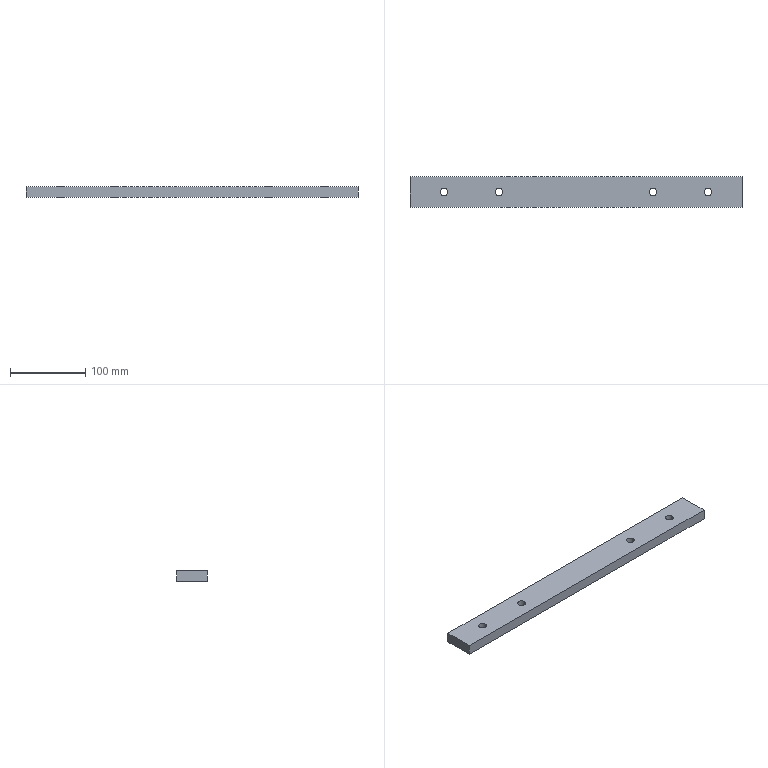Part | SolidWorks | features 3DProfileFeature 1, Extrusion 1, HoleWzd 1 | 1 solid | 14 faces | box 440 x 40 x 14 mm | volume 241824 mm3 | cylinder 8 | plane 6 | commonest cylinder face diameters 10.2 x8
STEP:
#1=CARTESIAN_POINT('',(50.1,20.,0.));
#2=VERTEX_POINT('',#1);
#3=CARTESIAN_POINT('',(39.9,20.,0.));
#4=VERTEX_POINT('',#3);
#5=CARTESIAN_POINT('',(45.,20.,0.));
#6=DIRECTION('',(0.,0.,-1.));
#7=DIRECTION('',(-1.,0.,0.));
#8=AXIS2_PLACEMENT_3D('',#5,#6,#7);
#9=CIRCLE('',#8,5.1);
#10=EDGE_CURVE('',#2,#4,#9,.T.);
#11=ORIENTED_EDGE('',*,*,#10,.T.);
#12=CARTESIAN_POINT('',(39.9,20.,14.));
#13=VERTEX_POINT('',#12);
#14=CARTESIAN_POINT('',(39.9,20.,14.));
#15=DIRECTION('',(0.,0.,1.));
#16=VECTOR('',#15,1000.);
#17=LINE('',#14,#16);
#18=EDGE_CURVE('',#4,#13,#17,.T.);
#19=ORIENTED_EDGE('',*,*,#18,.T.);
#20=CARTESIAN_POINT('',(50.1,20.,14.));
#21=VERTEX_POINT('',#20);
#22=CARTESIAN_POINT('',(45.,20.,14.));
#23=DIRECTION('',(0.,0.,1.));
#24=DIRECTION('',(1.,0.,0.));
#25=AXIS2_PLACEMENT_3D('',#22,#23,#24);
#26=CIRCLE('',#25,5.1);
#27=EDGE_CURVE('',#13,#21,#26,.T.);
#28=ORIENTED_EDGE('',*,*,#27,.T.);
#29=CARTESIAN_POINT('',(50.1,20.,14.));
#30=DIRECTION('',(0.,0.,1.));
#31=VECTOR('',#30,1000.);
#32=LINE('',#29,#31);
#33=EDGE_CURVE('',#2,#21,#32,.T.);
#34=ORIENTED_EDGE('',*,*,#33,.F.);
#35=EDGE_LOOP('',(#11,#19,#28,#34));
#36=FACE_OUTER_BOUND('',#35,.T.);
#37=CARTESIAN_POINT('',(45.,20.,14.));
#38=DIRECTION('',(0.,0.,1.));
#39=DIRECTION('',(1.,0.,0.));
#40=AXIS2_PLACEMENT_3D('',#37,#38,#39);
#41=CYLINDRICAL_SURFACE('',#40,5.1);
#42=ADVANCED_FACE('',(#36),#41,.F.);
#43=CARTESIAN_POINT('',(123.1,20.,0.));
#44=VERTEX_POINT('',#43);
#45=CARTESIAN_POINT('',(112.9,20.,0.));
#46=VERTEX_POINT('',#45);
#47=CARTESIAN_POINT('',(118.,20.,0.));
#48=DIRECTION('',(0.,0.,-1.));
#49=DIRECTION('',(-1.,0.,0.));
#50=AXIS2_PLACEMENT_3D('',#47,#48,#49);
#51=CIRCLE('',#50,5.1);
#52=EDGE_CURVE('',#44,#46,#51,.T.);
#53=ORIENTED_EDGE('',*,*,#52,.T.);
#54=CARTESIAN_POINT('',(112.9,20.,14.));
#55=VERTEX_POINT('',#54);
#56=CARTESIAN_POINT('',(112.9,20.,14.));
#57=DIRECTION('',(0.,0.,1.));
#58=VECTOR('',#57,1000.);
#59=LINE('',#56,#58);
#60=EDGE_CURVE('',#46,#55,#59,.T.);
#61=ORIENTED_EDGE('',*,*,#60,.T.);
#62=CARTESIAN_POINT('',(123.1,20.,14.));
#63=VERTEX_POINT('',#62);
#64=CARTESIAN_POINT('',(118.,20.,14.));
#65=DIRECTION('',(0.,0.,1.));
#66=DIRECTION('',(1.,0.,0.));
#67=AXIS2_PLACEMENT_3D('',#64,#65,#66);
#68=CIRCLE('',#67,5.1);
#69=EDGE_CURVE('',#55,#63,#68,.T.);
#70=ORIENTED_EDGE('',*,*,#69,.T.);
#71=CARTESIAN_POINT('',(123.1,20.,14.));
#72=DIRECTION('',(0.,0.,1.));
#73=VECTOR('',#72,1000.);
#74=LINE('',#71,#73);
#75=EDGE_CURVE('',#44,#63,#74,.T.);
#76=ORIENTED_EDGE('',*,*,#75,.F.);
#77=EDGE_LOOP('',(#53,#61,#70,#76));
#78=FACE_OUTER_BOUND('',#77,.T.);
#79=CARTESIAN_POINT('',(118.,20.,14.));
#80=DIRECTION('',(0.,0.,1.));
#81=DIRECTION('',(1.,0.,0.));
#82=AXIS2_PLACEMENT_3D('',#79,#80,#81);
#83=CYLINDRICAL_SURFACE('',#82,5.1);
#84=ADVANCED_FACE('',(#78),#83,.F.);
#85=CARTESIAN_POINT('',(400.1,20.,0.));
#86=VERTEX_POINT('',#85);
#87=CARTESIAN_POINT('',(389.9,20.,0.));
#88=VERTEX_POINT('',#87);
#89=CARTESIAN_POINT('',(395.,20.,0.));
#90=DIRECTION('',(0.,0.,-1.));
#91=DIRECTION('',(-1.,0.,0.));
#92=AXIS2_PLACEMENT_3D('',#89,#90,#91);
#93=CIRCLE('',#92,5.1);
#94=EDGE_CURVE('',#86,#88,#93,.T.);
#95=ORIENTED_EDGE('',*,*,#94,.T.);
#96=CARTESIAN_POINT('',(389.9,20.,14.));
#97=VERTEX_POINT('',#96);
#98=CARTESIAN_POINT('',(389.9,20.,14.));
#99=DIRECTION('',(0.,0.,1.));
#100=VECTOR('',#99,1000.);
#101=LINE('',#98,#100);
#102=EDGE_CURVE('',#88,#97,#101,.T.);
#103=ORIENTED_EDGE('',*,*,#102,.T.);
#104=CARTESIAN_POINT('',(400.1,20.,14.));
#105=VERTEX_POINT('',#104);
#106=CARTESIAN_POINT('',(395.,20.,14.));
#107=DIRECTION('',(0.,0.,1.));
#108=DIRECTION('',(1.,0.,0.));
#109=AXIS2_PLACEMENT_3D('',#106,#107,#108);
#110=CIRCLE('',#109,5.1);
#111=EDGE_CURVE('',#97,#105,#110,.T.);
#112=ORIENTED_EDGE('',*,*,#111,.T.);
#113=CARTESIAN_POINT('',(400.1,20.,14.));
#114=DIRECTION('',(0.,0.,1.));
#115=VECTOR('',#114,1000.);
#116=LINE('',#113,#115);
#117=EDGE_CURVE('',#86,#105,#116,.T.);
#118=ORIENTED_EDGE('',*,*,#117,.F.);
#119=EDGE_LOOP('',(#95,#103,#112,#118));
#120=FACE_OUTER_BOUND('',#119,.T.);
#121=CARTESIAN_POINT('',(395.,20.,14.));
#122=DIRECTION('',(0.,0.,1.));
#123=DIRECTION('',(1.,0.,0.));
#124=AXIS2_PLACEMENT_3D('',#121,#122,#123);
#125=CYLINDRICAL_SURFACE('',#124,5.1);
#126=ADVANCED_FACE('',(#120),#125,.F.);
#127=CARTESIAN_POINT('',(327.1,20.,0.));
#128=VERTEX_POINT('',#127);
#129=CARTESIAN_POINT('',(316.9,20.,0.));
#130=VERTEX_POINT('',#129);
#131=CARTESIAN_POINT('',(322.,20.,0.));
#132=DIRECTION('',(0.,0.,-1.));
#133=DIRECTION('',(-1.,0.,0.));
#134=AXIS2_PLACEMENT_3D('',#131,#132,#133);
#135=CIRCLE('',#134,5.1);
#136=EDGE_CURVE('',#128,#130,#135,.T.);
#137=ORIENTED_EDGE('',*,*,#136,.T.);
#138=CARTESIAN_POINT('',(316.9,20.,14.));
#139=VERTEX_POINT('',#138);
#140=CARTESIAN_POINT('',(316.9,20.,14.));
#141=DIRECTION('',(0.,0.,1.));
#142=VECTOR('',#141,1000.);
#143=LINE('',#140,#142);
#144=EDGE_CURVE('',#130,#139,#143,.T.);
#145=ORIENTED_EDGE('',*,*,#144,.T.);
#146=CARTESIAN_POINT('',(327.1,20.,14.));
#147=VERTEX_POINT('',#146);
#148=CARTESIAN_POINT('',(322.,20.,14.));
#149=DIRECTION('',(0.,0.,1.));
#150=DIRECTION('',(1.,0.,0.));
#151=AXIS2_PLACEMENT_3D('',#148,#149,#150);
#152=CIRCLE('',#151,5.1);
#153=EDGE_CURVE('',#139,#147,#152,.T.);
#154=ORIENTED_EDGE('',*,*,#153,.T.);
#155=CARTESIAN_POINT('',(327.1,20.,14.));
#156=DIRECTION('',(0.,0.,1.));
#157=VECTOR('',#156,1000.);
#158=LINE('',#155,#157);
#159=EDGE_CURVE('',#128,#147,#158,.T.);
#160=ORIENTED_EDGE('',*,*,#159,.F.);
#161=EDGE_LOOP('',(#137,#145,#154,#160));
#162=FACE_OUTER_BOUND('',#161,.T.);
#163=CARTESIAN_POINT('',(322.,20.,14.));
#164=DIRECTION('',(0.,0.,1.));
#165=DIRECTION('',(1.,0.,0.));
#166=AXIS2_PLACEMENT_3D('',#163,#164,#165);
#167=CYLINDRICAL_SURFACE('',#166,5.1);
#168=ADVANCED_FACE('',(#162),#167,.F.);
#169=CARTESIAN_POINT('',(0.,40.,0.));
#170=VERTEX_POINT('',#169);
#171=CARTESIAN_POINT('',(0.,0.,0.));
#172=VERTEX_POINT('',#171);
#173=CARTESIAN_POINT('',(0.,0.,0.));
#174=DIRECTION('',(0.,-1.,0.));
#175=VECTOR('',#174,1000.);
#176=LINE('',#173,#175);
#177=EDGE_CURVE('',#170,#172,#176,.T.);
#178=ORIENTED_EDGE('',*,*,#177,.T.);
#179=CARTESIAN_POINT('',(0.,0.,14.));
#180=VERTEX_POINT('',#179);
#181=CARTESIAN_POINT('',(0.,0.,14.));
#182=DIRECTION('',(0.,0.,-1.));
#183=VECTOR('',#182,1000.);
#184=LINE('',#181,#183);
#185=EDGE_CURVE('',#180,#172,#184,.T.);
#186=ORIENTED_EDGE('',*,*,#185,.F.);
#187=CARTESIAN_POINT('',(0.,40.,14.));
#188=VERTEX_POINT('',#187);
#189=CARTESIAN_POINT('',(0.,0.,14.));
#190=DIRECTION('',(0.,-1.,0.));
#191=VECTOR('',#190,1000.);
#192=LINE('',#189,#191);
#193=EDGE_CURVE('',#188,#180,#192,.T.);
#194=ORIENTED_EDGE('',*,*,#193,.F.);
#195=CARTESIAN_POINT('',(0.,40.,14.));
#196=DIRECTION('',(0.,0.,-1.));
#197=VECTOR('',#196,1000.);
#198=LINE('',#195,#197);
#199=EDGE_CURVE('',#188,#170,#198,.T.);
#200=ORIENTED_EDGE('',*,*,#199,.T.);
#201=EDGE_LOOP('',(#178,#186,#194,#200));
#202=FACE_OUTER_BOUND('',#201,.T.);
#203=CARTESIAN_POINT('',(0.,0.,14.));
#204=DIRECTION('',(1.,0.,0.));
#205=DIRECTION('',(0.,0.,-1.));
#206=AXIS2_PLACEMENT_3D('',#203,#204,#205);
#207=PLANE('',#206);
#208=ADVANCED_FACE('',(#202),#207,.F.);
#209=CARTESIAN_POINT('',(440.,0.,0.));
#210=VERTEX_POINT('',#209);
#211=CARTESIAN_POINT('',(0.,0.,0.));
#212=DIRECTION('',(1.,0.,0.));
#213=VECTOR('',#212,1000.);
#214=LINE('',#211,#213);
#215=EDGE_CURVE('',#172,#210,#214,.T.);
#216=ORIENTED_EDGE('',*,*,#215,.T.);
#217=CARTESIAN_POINT('',(440.,0.,14.));
#218=VERTEX_POINT('',#217);
#219=CARTESIAN_POINT('',(440.,0.,14.));
#220=DIRECTION('',(0.,0.,-1.));
#221=VECTOR('',#220,1000.);
#222=LINE('',#219,#221);
#223=EDGE_CURVE('',#218,#210,#222,.T.);
#224=ORIENTED_EDGE('',*,*,#223,.F.);
#225=CARTESIAN_POINT('',(0.,0.,14.));
#226=DIRECTION('',(1.,0.,0.));
#227=VECTOR('',#226,1000.);
#228=LINE('',#225,#227);
#229=EDGE_CURVE('',#180,#218,#228,.T.);
#230=ORIENTED_EDGE('',*,*,#229,.F.);
#231=ORIENTED_EDGE('',*,*,#185,.T.);
#232=EDGE_LOOP('',(#216,#224,#230,#231));
#233=FACE_OUTER_BOUND('',#232,.T.);
#234=CARTESIAN_POINT('',(0.,0.,14.));
#235=DIRECTION('',(0.,1.,0.));
#236=DIRECTION('',(0.,0.,1.));
#237=AXIS2_PLACEMENT_3D('',#234,#235,#236);
#238=PLANE('',#237);
#239=ADVANCED_FACE('',(#233),#238,.F.);
#240=CARTESIAN_POINT('',(440.,40.,0.));
#241=VERTEX_POINT('',#240);
#242=CARTESIAN_POINT('',(440.,0.,0.));
#243=DIRECTION('',(0.,1.,0.));
#244=VECTOR('',#243,1000.);
#245=LINE('',#242,#244);
#246=EDGE_CURVE('',#210,#241,#245,.T.);
#247=ORIENTED_EDGE('',*,*,#246,.T.);
#248=CARTESIAN_POINT('',(440.,40.,14.));
#249=VERTEX_POINT('',#248);
#250=CARTESIAN_POINT('',(440.,40.,14.));
#251=DIRECTION('',(0.,0.,-1.));
#252=VECTOR('',#251,1000.);
#253=LINE('',#250,#252);
#254=EDGE_CURVE('',#249,#241,#253,.T.);
#255=ORIENTED_EDGE('',*,*,#254,.F.);
#256=CARTESIAN_POINT('',(440.,0.,14.));
#257=DIRECTION('',(0.,1.,0.));
#258=VECTOR('',#257,1000.);
#259=LINE('',#256,#258);
#260=EDGE_CURVE('',#218,#249,#259,.T.);
#261=ORIENTED_EDGE('',*,*,#260,.F.);
#262=ORIENTED_EDGE('',*,*,#223,.T.);
#263=EDGE_LOOP('',(#247,#255,#261,#262));
#264=FACE_OUTER_BOUND('',#263,.T.);
#265=CARTESIAN_POINT('',(440.,0.,14.));
#266=DIRECTION('',(-1.,0.,0.));
#267=DIRECTION('',(0.,0.,1.));
#268=AXIS2_PLACEMENT_3D('',#265,#266,#267);
#269=PLANE('',#268);
#270=ADVANCED_FACE('',(#264),#269,.F.);
#271=CARTESIAN_POINT('',(0.,40.,0.));
#272=DIRECTION('',(-1.,0.,0.));
#273=VECTOR('',#272,1000.);
#274=LINE('',#271,#273);
#275=EDGE_CURVE('',#241,#170,#274,.T.);
#276=ORIENTED_EDGE('',*,*,#275,.T.);
#277=ORIENTED_EDGE('',*,*,#199,.F.);
#278=CARTESIAN_POINT('',(0.,40.,14.));
#279=DIRECTION('',(-1.,0.,0.));
#280=VECTOR('',#279,1000.);
#281=LINE('',#278,#280);
#282=EDGE_CURVE('',#249,#188,#281,.T.);
#283=ORIENTED_EDGE('',*,*,#282,.F.);
#284=ORIENTED_EDGE('',*,*,#254,.T.);
#285=EDGE_LOOP('',(#276,#277,#283,#284));
#286=FACE_OUTER_BOUND('',#285,.T.);
#287=CARTESIAN_POINT('',(0.,40.,14.));
#288=DIRECTION('',(0.,-1.,0.));
#289=DIRECTION('',(0.,0.,-1.));
#290=AXIS2_PLACEMENT_3D('',#287,#288,#289);
#291=PLANE('',#290);
#292=ADVANCED_FACE('',(#286),#291,.F.);
#293=CARTESIAN_POINT('',(45.,20.,14.));
#294=DIRECTION('',(0.,0.,1.));
#295=DIRECTION('',(1.,0.,0.));
#296=AXIS2_PLACEMENT_3D('',#293,#294,#295);
#297=CIRCLE('',#296,5.1);
#298=EDGE_CURVE('',#21,#13,#297,.T.);
#299=ORIENTED_EDGE('',*,*,#298,.F.);
#300=ORIENTED_EDGE('',*,*,#27,.F.);
#301=EDGE_LOOP('',(#299,#300));
#302=FACE_BOUND('',#301,.T.);
#303=CARTESIAN_POINT('',(118.,20.,14.));
#304=DIRECTION('',(0.,0.,1.));
#305=DIRECTION('',(1.,0.,0.));
#306=AXIS2_PLACEMENT_3D('',#303,#304,#305);
#307=CIRCLE('',#306,5.1);
#308=EDGE_CURVE('',#63,#55,#307,.T.);
#309=ORIENTED_EDGE('',*,*,#308,.F.);
#310=ORIENTED_EDGE('',*,*,#69,.F.);
#311=EDGE_LOOP('',(#309,#310));
#312=FACE_BOUND('',#311,.T.);
#313=CARTESIAN_POINT('',(395.,20.,14.));
#314=DIRECTION('',(0.,0.,1.));
#315=DIRECTION('',(1.,0.,0.));
#316=AXIS2_PLACEMENT_3D('',#313,#314,#315);
#317=CIRCLE('',#316,5.1);
#318=EDGE_CURVE('',#105,#97,#317,.T.);
#319=ORIENTED_EDGE('',*,*,#318,.F.);
#320=ORIENTED_EDGE('',*,*,#111,.F.);
#321=EDGE_LOOP('',(#319,#320));
#322=FACE_BOUND('',#321,.T.);
#323=CARTESIAN_POINT('',(322.,20.,14.));
#324=DIRECTION('',(0.,0.,1.));
#325=DIRECTION('',(1.,0.,0.));
#326=AXIS2_PLACEMENT_3D('',#323,#324,#325);
#327=CIRCLE('',#326,5.1);
#328=EDGE_CURVE('',#147,#139,#327,.T.);
#329=ORIENTED_EDGE('',*,*,#328,.F.);
#330=ORIENTED_EDGE('',*,*,#153,.F.);
#331=EDGE_LOOP('',(#329,#330));
#332=FACE_BOUND('',#331,.T.);
#333=ORIENTED_EDGE('',*,*,#193,.T.);
#334=ORIENTED_EDGE('',*,*,#229,.T.);
#335=ORIENTED_EDGE('',*,*,#260,.T.);
#336=ORIENTED_EDGE('',*,*,#282,.T.);
#337=EDGE_LOOP('',(#333,#334,#335,#336));
#338=FACE_OUTER_BOUND('',#337,.T.);
#339=CARTESIAN_POINT('',(0.,0.,14.));
#340=DIRECTION('',(0.,0.,-1.));
#341=DIRECTION('',(-1.,0.,0.));
#342=AXIS2_PLACEMENT_3D('',#339,#340,#341);
#343=PLANE('',#342);
#344=ADVANCED_FACE('',(#302,#312,#322,#332,#338),#343,.F.);
#345=ORIENTED_EDGE('',*,*,#10,.F.);
#346=CARTESIAN_POINT('',(45.,20.,0.));
#347=DIRECTION('',(0.,0.,-1.));
#348=DIRECTION('',(-1.,0.,0.));
#349=AXIS2_PLACEMENT_3D('',#346,#347,#348);
#350=CIRCLE('',#349,5.1);
#351=EDGE_CURVE('',#4,#2,#350,.T.);
#352=ORIENTED_EDGE('',*,*,#351,.F.);
#353=EDGE_LOOP('',(#345,#352));
#354=FACE_BOUND('',#353,.T.);
#355=ORIENTED_EDGE('',*,*,#52,.F.);
#356=CARTESIAN_POINT('',(118.,20.,0.));
#357=DIRECTION('',(0.,0.,-1.));
#358=DIRECTION('',(-1.,0.,0.));
#359=AXIS2_PLACEMENT_3D('',#356,#357,#358);
#360=CIRCLE('',#359,5.1);
#361=EDGE_CURVE('',#46,#44,#360,.T.);
#362=ORIENTED_EDGE('',*,*,#361,.F.);
#363=EDGE_LOOP('',(#355,#362));
#364=FACE_BOUND('',#363,.T.);
#365=ORIENTED_EDGE('',*,*,#94,.F.);
#366=CARTESIAN_POINT('',(395.,20.,0.));
#367=DIRECTION('',(0.,0.,-1.));
#368=DIRECTION('',(-1.,0.,0.));
#369=AXIS2_PLACEMENT_3D('',#366,#367,#368);
#370=CIRCLE('',#369,5.1);
#371=EDGE_CURVE('',#88,#86,#370,.T.);
#372=ORIENTED_EDGE('',*,*,#371,.F.);
#373=EDGE_LOOP('',(#365,#372));
#374=FACE_BOUND('',#373,.T.);
#375=ORIENTED_EDGE('',*,*,#136,.F.);
#376=CARTESIAN_POINT('',(322.,20.,0.));
#377=DIRECTION('',(0.,0.,-1.));
#378=DIRECTION('',(-1.,0.,0.));
#379=AXIS2_PLACEMENT_3D('',#376,#377,#378);
#380=CIRCLE('',#379,5.1);
#381=EDGE_CURVE('',#130,#128,#380,.T.);
#382=ORIENTED_EDGE('',*,*,#381,.F.);
#383=EDGE_LOOP('',(#375,#382));
#384=FACE_BOUND('',#383,.T.);
#385=ORIENTED_EDGE('',*,*,#177,.F.);
#386=ORIENTED_EDGE('',*,*,#275,.F.);
#387=ORIENTED_EDGE('',*,*,#246,.F.);
#388=ORIENTED_EDGE('',*,*,#215,.F.);
#389=EDGE_LOOP('',(#385,#386,#387,#388));
#390=FACE_OUTER_BOUND('',#389,.T.);
#391=CARTESIAN_POINT('',(0.,0.,0.));
#392=DIRECTION('',(0.,0.,-1.));
#393=DIRECTION('',(-1.,0.,0.));
#394=AXIS2_PLACEMENT_3D('',#391,#392,#393);
#395=PLANE('',#394);
#396=ADVANCED_FACE('',(#354,#364,#374,#384,#390),#395,.T.);
#397=ORIENTED_EDGE('',*,*,#144,.F.);
#398=ORIENTED_EDGE('',*,*,#381,.T.);
#399=ORIENTED_EDGE('',*,*,#159,.T.);
#400=ORIENTED_EDGE('',*,*,#328,.T.);
#401=EDGE_LOOP('',(#397,#398,#399,#400));
#402=FACE_OUTER_BOUND('',#401,.T.);
#403=CARTESIAN_POINT('',(322.,20.,14.));
#404=DIRECTION('',(0.,0.,1.));
#405=DIRECTION('',(1.,0.,0.));
#406=AXIS2_PLACEMENT_3D('',#403,#404,#405);
#407=CYLINDRICAL_SURFACE('',#406,5.1);
#408=ADVANCED_FACE('',(#402),#407,.F.);
#409=ORIENTED_EDGE('',*,*,#102,.F.);
#410=ORIENTED_EDGE('',*,*,#371,.T.);
#411=ORIENTED_EDGE('',*,*,#117,.T.);
#412=ORIENTED_EDGE('',*,*,#318,.T.);
#413=EDGE_LOOP('',(#409,#410,#411,#412));
#414=FACE_OUTER_BOUND('',#413,.T.);
#415=CARTESIAN_POINT('',(395.,20.,14.));
#416=DIRECTION('',(0.,0.,1.));
#417=DIRECTION('',(1.,0.,0.));
#418=AXIS2_PLACEMENT_3D('',#415,#416,#417);
#419=CYLINDRICAL_SURFACE('',#418,5.1);
#420=ADVANCED_FACE('',(#414),#419,.F.);
#421=ORIENTED_EDGE('',*,*,#60,.F.);
#422=ORIENTED_EDGE('',*,*,#361,.T.);
#423=ORIENTED_EDGE('',*,*,#75,.T.);
#424=ORIENTED_EDGE('',*,*,#308,.T.);
#425=EDGE_LOOP('',(#421,#422,#423,#424));
#426=FACE_OUTER_BOUND('',#425,.T.);
#427=CARTESIAN_POINT('',(118.,20.,14.));
#428=DIRECTION('',(0.,0.,1.));
#429=DIRECTION('',(1.,0.,0.));
#430=AXIS2_PLACEMENT_3D('',#427,#428,#429);
#431=CYLINDRICAL_SURFACE('',#430,5.1);
#432=ADVANCED_FACE('',(#426),#431,.F.);
#433=ORIENTED_EDGE('',*,*,#18,.F.);
#434=ORIENTED_EDGE('',*,*,#351,.T.);
#435=ORIENTED_EDGE('',*,*,#33,.T.);
#436=ORIENTED_EDGE('',*,*,#298,.T.);
#437=EDGE_LOOP('',(#433,#434,#435,#436));
#438=FACE_OUTER_BOUND('',#437,.T.);
#439=CARTESIAN_POINT('',(45.,20.,14.));
#440=DIRECTION('',(0.,0.,1.));
#441=DIRECTION('',(1.,0.,0.));
#442=AXIS2_PLACEMENT_3D('',#439,#440,#441);
#443=CYLINDRICAL_SURFACE('',#442,5.1);
#444=ADVANCED_FACE('',(#438),#443,.F.);
#445=CLOSED_SHELL('',(#42,#84,#126,#168,#208,#239,#270,#292,#344,#396,#408,#420,#432,#444));
#446=MANIFOLD_SOLID_BREP('',#445);
#447=CARTESIAN_POINT('',(0.,0.,0.));
#448=DIRECTION('',(0.,0.,1.));
#449=DIRECTION('',(1.,0.,0.));
#450=AXIS2_PLACEMENT_3D('',#447,#448,#449);
#451=(LENGTH_UNIT()NAMED_UNIT(*)SI_UNIT(.MILLI.,.METRE.));
#452=UNCERTAINTY_MEASURE_WITH_UNIT(LENGTH_MEASURE(0.00001),#451,'','');
#453=(NAMED_UNIT(*)PLANE_ANGLE_UNIT()SI_UNIT($,.RADIAN.));
#454=(NAMED_UNIT(*)SI_UNIT($,.STERADIAN.)SOLID_ANGLE_UNIT());
#455=(GEOMETRIC_REPRESENTATION_CONTEXT(3)GLOBAL_UNCERTAINTY_ASSIGNED_CONTEXT((#452))GLOBAL_UNIT_ASSIGNED_CONTEXT((#451,#453,#454))REPRESENTATION_CONTEXT('',''));
#456=ADVANCED_BREP_SHAPE_REPRESENTATION('',(#446,#450),#455);